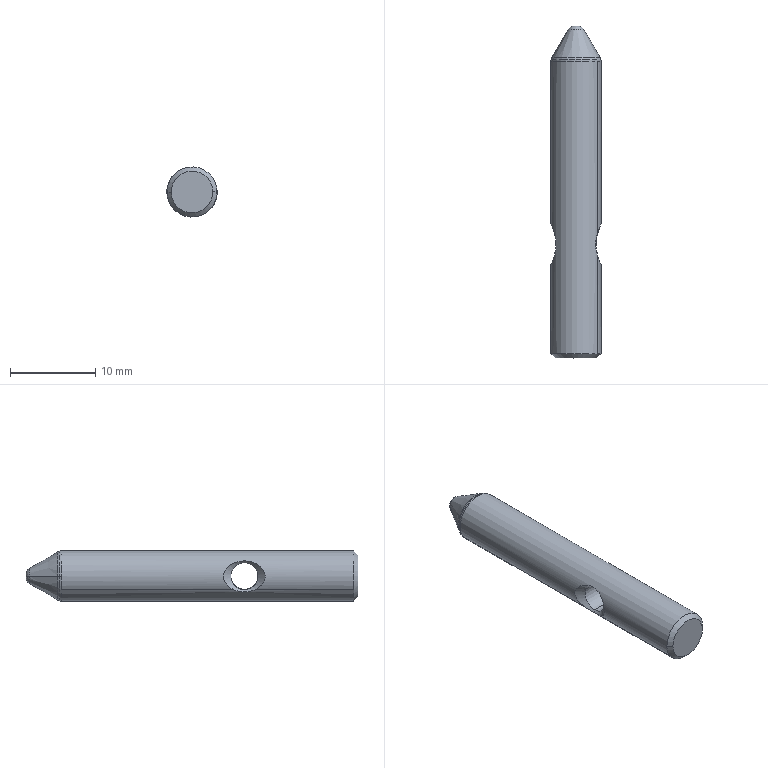Part | NX | features solid 2 | 1 solid | 20 faces | box 5.9 x 39 x 5.9 mm | volume 952.663 mm3 | cone 8 | cylinder 4 | torus 4 | spline 2 | plane 2 | commonest cylinder face diameters 3.2 x2 5.9 x2
STEP:
#1=CARTESIAN_POINT('',(286.395,55.027,28.705));
#2=VERTEX_POINT('',#1);
#3=CARTESIAN_POINT('',(286.206,53.764,28.965));
#4=VERTEX_POINT('',#3);
#5=CARTESIAN_POINT('',(286.395,55.027,28.705));
#6=CARTESIAN_POINT('',(286.283,54.637,28.879));
#7=CARTESIAN_POINT('',(286.206,54.207,28.965));
#8=CARTESIAN_POINT('',(286.206,53.764,28.965));
#9=B_SPLINE_CURVE_WITH_KNOTS('',3,(#5,#6,#7,#8),.UNSPECIFIED.,.F.,.F.,(4,4),(0.,0.001307),.UNSPECIFIED.);
#10=EDGE_CURVE('',#2,#4,#9,.T.);
#11=ORIENTED_EDGE('',*,*,#10,.F.);
#12=CARTESIAN_POINT('',(286.395,75.273,28.705));
#13=VERTEX_POINT('',#12);
#14=CARTESIAN_POINT('',(286.395,51.692,28.705));
#15=DIRECTION('',(0.,-1.,0.));
#16=VECTOR('',#15,1000.);
#17=LINE('',#14,#16);
#18=EDGE_CURVE('',#13,#2,#17,.T.);
#19=ORIENTED_EDGE('',*,*,#18,.F.);
#20=CARTESIAN_POINT('',(280.971,75.273,27.044));
#21=VERTEX_POINT('',#20);
#22=CARTESIAN_POINT('',(283.92,75.273,27.1));
#23=DIRECTION('',(0.,1.,0.));
#24=DIRECTION('',(-0.9998,0.,-0.01902));
#25=AXIS2_PLACEMENT_3D('',#22,#23,#24);
#26=CIRCLE('',#25,2.95);
#27=EDGE_CURVE('',#21,#13,#26,.T.);
#28=ORIENTED_EDGE('',*,*,#27,.F.);
#29=CARTESIAN_POINT('',(281.445,75.273,25.495));
#30=VERTEX_POINT('',#29);
#31=CARTESIAN_POINT('',(283.92,75.273,27.1));
#32=DIRECTION('',(0.,1.,0.));
#33=DIRECTION('',(-0.8391,0.,-0.5441));
#34=AXIS2_PLACEMENT_3D('',#31,#32,#33);
#35=CIRCLE('',#34,2.95);
#36=EDGE_CURVE('',#30,#21,#35,.T.);
#37=ORIENTED_EDGE('',*,*,#36,.F.);
#38=CARTESIAN_POINT('',(281.445,55.027,25.495));
#39=VERTEX_POINT('',#38);
#40=CARTESIAN_POINT('',(281.445,75.273,25.495));
#41=DIRECTION('',(0.000000064,-1.,-0.000000369));
#42=VECTOR('',#41,1000.);
#43=LINE('',#40,#42);
#44=EDGE_CURVE('',#39,#30,#43,.F.);
#45=ORIENTED_EDGE('',*,*,#44,.F.);
#46=CARTESIAN_POINT('',(281.12,55.909,26.17));
#47=VERTEX_POINT('',#46);
#48=CARTESIAN_POINT('',(281.12,55.909,26.17));
#49=CARTESIAN_POINT('',(281.221,55.681,25.866));
#50=CARTESIAN_POINT('',(281.345,55.373,25.649));
#51=CARTESIAN_POINT('',(281.445,55.027,25.495));
#52=B_SPLINE_CURVE_WITH_KNOTS('',3,(#48,#49,#50,#51),.UNSPECIFIED.,.F.,.F.,(4,4),(0.,0.001162),.UNSPECIFIED.);
#53=EDGE_CURVE('',#47,#39,#52,.T.);
#54=ORIENTED_EDGE('',*,*,#53,.F.);
#55=CARTESIAN_POINT('',(281.565,53.764,28.876));
#56=VERTEX_POINT('',#55);
#57=CARTESIAN_POINT('',(281.565,53.764,28.876));
#58=CARTESIAN_POINT('',(281.565,54.133,28.876));
#59=CARTESIAN_POINT('',(281.463,54.856,28.747));
#60=CARTESIAN_POINT('',(281.147,55.78,28.215));
#61=CARTESIAN_POINT('',(280.898,56.363,27.214));
#62=CARTESIAN_POINT('',(281.025,56.124,26.457));
#63=CARTESIAN_POINT('',(281.12,55.909,26.17));
#64=B_SPLINE_CURVE_WITH_KNOTS('',3,(#57,#58,#59,#60,#61,#62,#63),.UNSPECIFIED.,.F.,.F.,(4,1,1,1,4),(0.,0.001091,0.002181,0.003272,0.004362),.UNSPECIFIED.);
#65=EDGE_CURVE('',#56,#47,#64,.T.);
#66=ORIENTED_EDGE('',*,*,#65,.F.);
#67=CARTESIAN_POINT('',(281.445,52.501,25.495));
#68=VERTEX_POINT('',#67);
#69=CARTESIAN_POINT('',(281.445,52.501,25.495));
#70=CARTESIAN_POINT('',(281.326,52.089,25.678));
#71=CARTESIAN_POINT('',(281.091,51.538,26.09));
#72=CARTESIAN_POINT('',(280.941,51.249,27.003));
#73=CARTESIAN_POINT('',(281.033,51.486,27.938));
#74=CARTESIAN_POINT('',(281.399,52.389,28.676));
#75=CARTESIAN_POINT('',(281.565,53.298,28.876));
#76=CARTESIAN_POINT('',(281.565,53.764,28.876));
#77=B_SPLINE_CURVE_WITH_KNOTS('',3,(#69,#70,#71,#72,#73,#74,#75,#76),.UNSPECIFIED.,.F.,.F.,(4,1,1,1,1,4),(0.000000001,0.001379,0.002068,0.002758,0.004136,0.005515),.UNSPECIFIED.);
#78=EDGE_CURVE('',#68,#56,#77,.T.);
#79=ORIENTED_EDGE('',*,*,#78,.F.);
#80=CARTESIAN_POINT('',(281.445,40.924,25.495));
#81=VERTEX_POINT('',#80);
#82=CARTESIAN_POINT('',(281.445,52.501,25.495));
#83=DIRECTION('',(0.000000047,-1.,0.000000146));
#84=VECTOR('',#83,1000.);
#85=LINE('',#82,#84);
#86=EDGE_CURVE('',#81,#68,#85,.F.);
#87=ORIENTED_EDGE('',*,*,#86,.F.);
#88=CARTESIAN_POINT('',(280.971,40.924,27.044));
#89=VERTEX_POINT('',#88);
#90=CARTESIAN_POINT('',(283.92,40.924,27.1));
#91=DIRECTION('',(0.,-1.,0.));
#92=DIRECTION('',(-0.9998,0.,-0.01902));
#93=AXIS2_PLACEMENT_3D('',#90,#91,#92);
#94=CIRCLE('',#93,2.95);
#95=EDGE_CURVE('',#89,#81,#94,.T.);
#96=ORIENTED_EDGE('',*,*,#95,.F.);
#97=CARTESIAN_POINT('',(286.395,40.924,28.705));
#98=VERTEX_POINT('',#97);
#99=CARTESIAN_POINT('',(283.92,40.924,27.1));
#100=DIRECTION('',(0.,-1.,0.));
#101=DIRECTION('',(0.8391,0.,0.5441));
#102=AXIS2_PLACEMENT_3D('',#99,#100,#101);
#103=CIRCLE('',#102,2.95);
#104=EDGE_CURVE('',#98,#89,#103,.T.);
#105=ORIENTED_EDGE('',*,*,#104,.F.);
#106=CARTESIAN_POINT('',(286.395,52.501,28.705));
#107=VERTEX_POINT('',#106);
#108=CARTESIAN_POINT('',(286.395,52.501,28.705));
#109=CARTESIAN_POINT('',(286.395,48.642,28.705));
#110=CARTESIAN_POINT('',(286.395,44.783,28.705));
#111=CARTESIAN_POINT('',(286.395,40.924,28.705));
#112=B_SPLINE_CURVE_WITH_KNOTS('',3,(#108,#109,#110,#111),.UNSPECIFIED.,.F.,.F.,(4,4),(0.,1.),.UNSPECIFIED.);
#113=EDGE_CURVE('',#107,#98,#112,.T.);
#114=ORIENTED_EDGE('',*,*,#113,.F.);
#115=CARTESIAN_POINT('',(286.206,53.764,28.965));
#116=CARTESIAN_POINT('',(286.206,53.322,28.965));
#117=CARTESIAN_POINT('',(286.283,52.891,28.878));
#118=CARTESIAN_POINT('',(286.395,52.501,28.705));
#119=B_SPLINE_CURVE_WITH_KNOTS('',3,(#115,#116,#117,#118),.UNSPECIFIED.,.F.,.F.,(4,4),(0.,0.001308),.UNSPECIFIED.);
#120=EDGE_CURVE('',#4,#107,#119,.T.);
#121=ORIENTED_EDGE('',*,*,#120,.F.);
#122=EDGE_LOOP('',(#11,#19,#28,#37,#45,#54,#66,#79,#87,#96,#105,#114,#121));
#123=FACE_BOUND('',#122,.T.);
#124=CARTESIAN_POINT('',(283.92,51.692,27.1));
#125=DIRECTION('',(0.,-1.,0.));
#126=DIRECTION('',(-0.8391,0.,-0.5441));
#127=AXIS2_PLACEMENT_3D('',#124,#125,#126);
#128=CYLINDRICAL_SURFACE('',#127,2.95);
#129=ADVANCED_FACE('',(#123),#128,.T.);
#130=CARTESIAN_POINT('',(286.05,53.764,25.54));
#131=VERTEX_POINT('',#130);
#132=CARTESIAN_POINT('',(286.275,53.764,25.324));
#133=VERTEX_POINT('',#132);
#134=CARTESIAN_POINT('',(286.05,53.764,25.54));
#135=DIRECTION('',(0.7204,-0.000000028,-0.6935));
#136=VECTOR('',#135,1000.);
#137=LINE('',#134,#136);
#138=EDGE_CURVE('',#131,#133,#137,.T.);
#139=ORIENTED_EDGE('',*,*,#138,.F.);
#140=CARTESIAN_POINT('',(285.989,53.764,28.74));
#141=VERTEX_POINT('',#140);
#142=CARTESIAN_POINT('',(286.02,53.764,27.14));
#143=DIRECTION('',(-0.9998,0.,-0.01902));
#144=DIRECTION('',(0.01902,0.,-0.9998));
#145=AXIS2_PLACEMENT_3D('',#142,#143,#144);
#146=CIRCLE('',#145,1.6);
#147=EDGE_CURVE('',#131,#141,#146,.T.);
#148=ORIENTED_EDGE('',*,*,#147,.T.);
#149=CARTESIAN_POINT('',(285.989,53.764,28.74));
#150=CARTESIAN_POINT('',(286.061,53.764,28.815));
#151=CARTESIAN_POINT('',(286.134,53.764,28.89));
#152=CARTESIAN_POINT('',(286.206,53.764,28.965));
#153=B_SPLINE_CURVE_WITH_KNOTS('',3,(#149,#150,#151,#152),.UNSPECIFIED.,.F.,.F.,(4,4),(0.,0.9998),.UNSPECIFIED.);
#154=EDGE_CURVE('',#4,#141,#153,.F.);
#155=ORIENTED_EDGE('',*,*,#154,.F.);
#156=ORIENTED_EDGE('',*,*,#120,.T.);
#157=CARTESIAN_POINT('',(286.395,52.501,28.705));
#158=CARTESIAN_POINT('',(286.514,52.089,28.521));
#159=CARTESIAN_POINT('',(286.749,51.537,28.109));
#160=CARTESIAN_POINT('',(286.899,51.249,27.197));
#161=CARTESIAN_POINT('',(286.807,51.487,26.262));
#162=CARTESIAN_POINT('',(286.441,52.389,25.524));
#163=CARTESIAN_POINT('',(286.275,53.298,25.324));
#164=CARTESIAN_POINT('',(286.275,53.764,25.324));
#165=B_SPLINE_CURVE_WITH_KNOTS('',3,(#157,#158,#159,#160,#161,#162,#163,#164),.UNSPECIFIED.,.F.,.F.,(4,1,1,1,1,4),(0.,0.001379,0.002068,0.002757,0.004136,0.005514),.UNSPECIFIED.);
#166=EDGE_CURVE('',#107,#133,#165,.T.);
#167=ORIENTED_EDGE('',*,*,#166,.T.);
#168=EDGE_LOOP('',(#139,#148,#155,#156,#167));
#169=FACE_BOUND('',#168,.T.);
#170=CARTESIAN_POINT('',(286.445,53.764,27.148));
#171=DIRECTION('',(0.9998,0.,0.01902));
#172=DIRECTION('',(0.01902,0.,-0.9998));
#173=AXIS2_PLACEMENT_3D('',#170,#171,#172);
#174=CONICAL_SURFACE('',#173,2.025,0.7854);
#175=ADVANCED_FACE('',(#169),#174,.F.);
#176=ORIENTED_EDGE('',*,*,#166,.F.);
#177=ORIENTED_EDGE('',*,*,#113,.T.);
#178=CARTESIAN_POINT('',(286.869,40.924,27.156));
#179=VERTEX_POINT('',#178);
#180=CARTESIAN_POINT('',(283.92,40.924,27.1));
#181=DIRECTION('',(0.,-1.,0.));
#182=DIRECTION('',(0.9998,0.,0.01902));
#183=AXIS2_PLACEMENT_3D('',#180,#181,#182);
#184=CIRCLE('',#183,2.95);
#185=EDGE_CURVE('',#179,#98,#184,.T.);
#186=ORIENTED_EDGE('',*,*,#185,.F.);
#187=CARTESIAN_POINT('',(283.92,40.924,27.1));
#188=DIRECTION('',(0.,-1.,0.));
#189=DIRECTION('',(-0.8391,0.,-0.5441));
#190=AXIS2_PLACEMENT_3D('',#187,#188,#189);
#191=CIRCLE('',#190,2.95);
#192=EDGE_CURVE('',#81,#179,#191,.T.);
#193=ORIENTED_EDGE('',*,*,#192,.F.);
#194=ORIENTED_EDGE('',*,*,#86,.T.);
#195=CARTESIAN_POINT('',(281.634,53.764,25.235));
#196=VERTEX_POINT('',#195);
#197=CARTESIAN_POINT('',(281.634,53.764,25.235));
#198=CARTESIAN_POINT('',(281.634,53.322,25.235));
#199=CARTESIAN_POINT('',(281.557,52.892,25.321));
#200=CARTESIAN_POINT('',(281.445,52.501,25.495));
#201=B_SPLINE_CURVE_WITH_KNOTS('',3,(#197,#198,#199,#200),.UNSPECIFIED.,.F.,.F.,(4,4),(0.,0.001307),.UNSPECIFIED.);
#202=EDGE_CURVE('',#196,#68,#201,.T.);
#203=ORIENTED_EDGE('',*,*,#202,.F.);
#204=CARTESIAN_POINT('',(281.445,55.027,25.495));
#205=CARTESIAN_POINT('',(281.557,54.637,25.321));
#206=CARTESIAN_POINT('',(281.634,54.207,25.235));
#207=CARTESIAN_POINT('',(281.634,53.764,25.235));
#208=B_SPLINE_CURVE_WITH_KNOTS('',3,(#204,#205,#206,#207),.UNSPECIFIED.,.F.,.F.,(4,4),(0.,0.001307),.UNSPECIFIED.);
#209=EDGE_CURVE('',#39,#196,#208,.T.);
#210=ORIENTED_EDGE('',*,*,#209,.F.);
#211=ORIENTED_EDGE('',*,*,#44,.T.);
#212=CARTESIAN_POINT('',(286.869,75.273,27.156));
#213=VERTEX_POINT('',#212);
#214=CARTESIAN_POINT('',(283.92,75.273,27.1));
#215=DIRECTION('',(0.,1.,0.));
#216=DIRECTION('',(0.9998,0.,0.01902));
#217=AXIS2_PLACEMENT_3D('',#214,#215,#216);
#218=CIRCLE('',#217,2.95);
#219=EDGE_CURVE('',#213,#30,#218,.T.);
#220=ORIENTED_EDGE('',*,*,#219,.F.);
#221=CARTESIAN_POINT('',(283.92,75.273,27.1));
#222=DIRECTION('',(0.,1.,0.));
#223=DIRECTION('',(0.8391,0.,0.5441));
#224=AXIS2_PLACEMENT_3D('',#221,#222,#223);
#225=CIRCLE('',#224,2.95);
#226=EDGE_CURVE('',#13,#213,#225,.T.);
#227=ORIENTED_EDGE('',*,*,#226,.F.);
#228=ORIENTED_EDGE('',*,*,#18,.T.);
#229=CARTESIAN_POINT('',(286.753,55.909,26.277));
#230=VERTEX_POINT('',#229);
#231=CARTESIAN_POINT('',(286.753,55.909,26.277));
#232=CARTESIAN_POINT('',(286.812,56.059,26.48));
#233=CARTESIAN_POINT('',(286.903,56.278,26.957));
#234=CARTESIAN_POINT('',(286.801,56.102,28.021));
#235=CARTESIAN_POINT('',(286.527,55.483,28.502));
#236=CARTESIAN_POINT('',(286.395,55.027,28.705));
#237=B_SPLINE_CURVE_WITH_KNOTS('',3,(#231,#232,#233,#234,#235,#236),.UNSPECIFIED.,.F.,.F.,(4,1,1,4),(0.,0.0007668,0.001534,0.003067),.UNSPECIFIED.);
#238=EDGE_CURVE('',#230,#2,#237,.T.);
#239=ORIENTED_EDGE('',*,*,#238,.F.);
#240=CARTESIAN_POINT('',(286.275,53.764,25.324));
#241=CARTESIAN_POINT('',(286.275,54.6,25.324));
#242=CARTESIAN_POINT('',(286.562,55.423,25.621));
#243=CARTESIAN_POINT('',(286.753,55.909,26.277));
#244=B_SPLINE_CURVE_WITH_KNOTS('',3,(#240,#241,#242,#243),.UNSPECIFIED.,.F.,.F.,(4,4),(0.,0.002472),.UNSPECIFIED.);
#245=EDGE_CURVE('',#133,#230,#244,.T.);
#246=ORIENTED_EDGE('',*,*,#245,.F.);
#247=EDGE_LOOP('',(#176,#177,#186,#193,#194,#203,#210,#211,#220,#227,#228,#239,#246));
#248=FACE_BOUND('',#247,.T.);
#249=CARTESIAN_POINT('',(283.92,51.692,27.1));
#250=DIRECTION('',(0.,-1.,0.));
#251=DIRECTION('',(-0.8391,0.,-0.5441));
#252=AXIS2_PLACEMENT_3D('',#249,#250,#251);
#253=CYLINDRICAL_SURFACE('',#252,2.95);
#254=ADVANCED_FACE('',(#248),#253,.T.);
#255=ORIENTED_EDGE('',*,*,#238,.T.);
#256=ORIENTED_EDGE('',*,*,#10,.T.);
#257=ORIENTED_EDGE('',*,*,#154,.T.);
#258=CARTESIAN_POINT('',(286.02,53.764,27.14));
#259=DIRECTION('',(-0.9998,0.,-0.01902));
#260=DIRECTION('',(-0.01902,0.,0.9998));
#261=AXIS2_PLACEMENT_3D('',#258,#259,#260);
#262=CIRCLE('',#261,1.6);
#263=EDGE_CURVE('',#141,#131,#262,.T.);
#264=ORIENTED_EDGE('',*,*,#263,.T.);
#265=ORIENTED_EDGE('',*,*,#138,.T.);
#266=ORIENTED_EDGE('',*,*,#245,.T.);
#267=EDGE_LOOP('',(#255,#256,#257,#264,#265,#266));
#268=FACE_BOUND('',#267,.T.);
#269=CARTESIAN_POINT('',(286.445,53.764,27.148));
#270=DIRECTION('',(0.9998,0.,0.01902));
#271=DIRECTION('',(0.01902,0.,-0.9998));
#272=AXIS2_PLACEMENT_3D('',#269,#270,#271);
#273=CONICAL_SURFACE('',#272,2.025,0.7854);
#274=ADVANCED_FACE('',(#268),#273,.F.);
#275=CARTESIAN_POINT('',(281.79,53.764,28.66));
#276=VERTEX_POINT('',#275);
#277=CARTESIAN_POINT('',(285.989,53.764,28.74));
#278=DIRECTION('',(-0.9998,0.,-0.01902));
#279=VECTOR('',#278,1000.);
#280=LINE('',#277,#279);
#281=EDGE_CURVE('',#141,#276,#280,.T.);
#282=ORIENTED_EDGE('',*,*,#281,.T.);
#283=CARTESIAN_POINT('',(281.851,53.764,25.46));
#284=VERTEX_POINT('',#283);
#285=CARTESIAN_POINT('',(281.82,53.764,27.06));
#286=DIRECTION('',(0.9998,0.,0.01902));
#287=DIRECTION('',(0.01902,0.,-0.9998));
#288=AXIS2_PLACEMENT_3D('',#285,#286,#287);
#289=CIRCLE('',#288,1.6);
#290=EDGE_CURVE('',#284,#276,#289,.T.);
#291=ORIENTED_EDGE('',*,*,#290,.F.);
#292=CARTESIAN_POINT('',(286.05,53.764,25.54));
#293=DIRECTION('',(-0.9998,0.,-0.01902));
#294=VECTOR('',#293,1000.);
#295=LINE('',#292,#294);
#296=EDGE_CURVE('',#284,#131,#295,.F.);
#297=ORIENTED_EDGE('',*,*,#296,.T.);
#298=ORIENTED_EDGE('',*,*,#263,.F.);
#299=EDGE_LOOP('',(#282,#291,#297,#298));
#300=FACE_BOUND('',#299,.T.);
#301=CARTESIAN_POINT('',(288.919,53.764,27.195));
#302=DIRECTION('',(-0.9998,0.,-0.01902));
#303=DIRECTION('',(-0.01902,0.,0.9998));
#304=AXIS2_PLACEMENT_3D('',#301,#302,#303);
#305=CYLINDRICAL_SURFACE('',#304,1.6);
#306=ADVANCED_FACE('',(#300),#305,.F.);
#307=ORIENTED_EDGE('',*,*,#296,.F.);
#308=CARTESIAN_POINT('',(281.82,53.764,27.06));
#309=DIRECTION('',(0.9998,0.,0.01902));
#310=DIRECTION('',(-0.01902,0.,0.9998));
#311=AXIS2_PLACEMENT_3D('',#308,#309,#310);
#312=CIRCLE('',#311,1.6);
#313=EDGE_CURVE('',#276,#284,#312,.T.);
#314=ORIENTED_EDGE('',*,*,#313,.F.);
#315=ORIENTED_EDGE('',*,*,#281,.F.);
#316=ORIENTED_EDGE('',*,*,#147,.F.);
#317=EDGE_LOOP('',(#307,#314,#315,#316));
#318=FACE_BOUND('',#317,.T.);
#319=CARTESIAN_POINT('',(288.919,53.764,27.195));
#320=DIRECTION('',(-0.9998,0.,-0.01902));
#321=DIRECTION('',(-0.01902,0.,0.9998));
#322=AXIS2_PLACEMENT_3D('',#319,#320,#321);
#323=CYLINDRICAL_SURFACE('',#322,1.6);
#324=ADVANCED_FACE('',(#318),#323,.F.);
#325=ORIENTED_EDGE('',*,*,#78,.T.);
#326=CARTESIAN_POINT('',(281.79,53.764,28.66));
#327=CARTESIAN_POINT('',(281.715,53.764,28.732));
#328=CARTESIAN_POINT('',(281.65,53.764,28.795));
#329=CARTESIAN_POINT('',(281.565,53.764,28.876));
#330=B_SPLINE_CURVE_WITH_KNOTS('',3,(#326,#327,#328,#329),.UNSPECIFIED.,.F.,.F.,(4,4),(0.,0.9999),.UNSPECIFIED.);
#331=EDGE_CURVE('',#276,#56,#330,.T.);
#332=ORIENTED_EDGE('',*,*,#331,.F.);
#333=ORIENTED_EDGE('',*,*,#313,.T.);
#334=CARTESIAN_POINT('',(281.851,53.764,25.46));
#335=CARTESIAN_POINT('',(281.779,53.764,25.385));
#336=CARTESIAN_POINT('',(281.706,53.764,25.31));
#337=CARTESIAN_POINT('',(281.634,53.764,25.235));
#338=B_SPLINE_CURVE_WITH_KNOTS('',3,(#334,#335,#336,#337),.UNSPECIFIED.,.F.,.F.,(4,4),(0.,0.9996),.UNSPECIFIED.);
#339=EDGE_CURVE('',#196,#284,#338,.F.);
#340=ORIENTED_EDGE('',*,*,#339,.F.);
#341=ORIENTED_EDGE('',*,*,#202,.T.);
#342=EDGE_LOOP('',(#325,#332,#333,#340,#341));
#343=FACE_BOUND('',#342,.T.);
#344=CARTESIAN_POINT('',(281.395,53.764,27.052));
#345=DIRECTION('',(-0.9998,0.,-0.01902));
#346=DIRECTION('',(-0.01902,0.,0.9998));
#347=AXIS2_PLACEMENT_3D('',#344,#345,#346);
#348=CONICAL_SURFACE('',#347,2.025,0.7854);
#349=ADVANCED_FACE('',(#343),#348,.F.);
#350=ORIENTED_EDGE('',*,*,#209,.T.);
#351=ORIENTED_EDGE('',*,*,#339,.T.);
#352=ORIENTED_EDGE('',*,*,#290,.T.);
#353=ORIENTED_EDGE('',*,*,#331,.T.);
#354=ORIENTED_EDGE('',*,*,#65,.T.);
#355=ORIENTED_EDGE('',*,*,#53,.T.);
#356=EDGE_LOOP('',(#350,#351,#352,#353,#354,#355));
#357=FACE_BOUND('',#356,.T.);
#358=CARTESIAN_POINT('',(281.395,53.764,27.052));
#359=DIRECTION('',(-0.9998,0.,-0.01902));
#360=DIRECTION('',(-0.01902,0.,0.9998));
#361=AXIS2_PLACEMENT_3D('',#358,#359,#360);
#362=CONICAL_SURFACE('',#361,2.025,0.7854);
#363=ADVANCED_FACE('',(#357),#362,.F.);
#364=ORIENTED_EDGE('',*,*,#226,.T.);
#365=CARTESIAN_POINT('',(286.842,75.48,27.156));
#366=VERTEX_POINT('',#365);
#367=CARTESIAN_POINT('',(286.07,75.273,27.141));
#368=DIRECTION('',(-0.01902,0.,0.9998));
#369=DIRECTION('',(0.9998,0.,0.01902));
#370=AXIS2_PLACEMENT_3D('',#367,#368,#369);
#371=CIRCLE('',#370,0.8);
#372=EDGE_CURVE('',#366,#213,#371,.F.);
#373=ORIENTED_EDGE('',*,*,#372,.F.);
#374=CARTESIAN_POINT('',(280.998,75.48,27.044));
#375=VERTEX_POINT('',#374);
#376=CARTESIAN_POINT('',(283.92,75.48,27.1));
#377=DIRECTION('',(0.,1.,0.));
#378=DIRECTION('',(-0.9998,0.,-0.01902));
#379=AXIS2_PLACEMENT_3D('',#376,#377,#378);
#380=CIRCLE('',#379,2.923);
#381=EDGE_CURVE('',#375,#366,#380,.T.);
#382=ORIENTED_EDGE('',*,*,#381,.F.);
#383=CARTESIAN_POINT('',(281.77,75.273,27.059));
#384=DIRECTION('',(0.01902,0.,-0.9998));
#385=DIRECTION('',(-0.9998,0.,-0.01902));
#386=AXIS2_PLACEMENT_3D('',#383,#384,#385);
#387=CIRCLE('',#386,0.8);
#388=EDGE_CURVE('',#21,#375,#387,.T.);
#389=ORIENTED_EDGE('',*,*,#388,.F.);
#390=ORIENTED_EDGE('',*,*,#27,.T.);
#391=EDGE_LOOP('',(#364,#373,#382,#389,#390));
#392=FACE_BOUND('',#391,.T.);
#393=CARTESIAN_POINT('',(283.92,75.273,27.1));
#394=DIRECTION('',(0.,1.,0.));
#395=DIRECTION('',(0.9998,0.,0.01902));
#396=AXIS2_PLACEMENT_3D('',#393,#394,#395);
#397=TOROIDAL_SURFACE('',#396,2.15,0.8);
#398=ADVANCED_FACE('',(#392),#397,.T.);
#399=ORIENTED_EDGE('',*,*,#36,.T.);
#400=ORIENTED_EDGE('',*,*,#388,.T.);
#401=CARTESIAN_POINT('',(283.92,75.48,27.1));
#402=DIRECTION('',(0.,1.,0.));
#403=DIRECTION('',(0.9998,0.,0.01902));
#404=AXIS2_PLACEMENT_3D('',#401,#402,#403);
#405=CIRCLE('',#404,2.923);
#406=EDGE_CURVE('',#366,#375,#405,.T.);
#407=ORIENTED_EDGE('',*,*,#406,.F.);
#408=ORIENTED_EDGE('',*,*,#372,.T.);
#409=ORIENTED_EDGE('',*,*,#219,.T.);
#410=EDGE_LOOP('',(#399,#400,#407,#408,#409));
#411=FACE_BOUND('',#410,.T.);
#412=CARTESIAN_POINT('',(283.92,75.273,27.1));
#413=DIRECTION('',(0.,1.,0.));
#414=DIRECTION('',(0.9998,0.,0.01902));
#415=AXIS2_PLACEMENT_3D('',#412,#413,#414);
#416=TOROIDAL_SURFACE('',#415,2.15,0.8);
#417=ADVANCED_FACE('',(#411),#416,.T.);
#418=CARTESIAN_POINT('',(286.762,75.673,27.154));
#419=VERTEX_POINT('',#418);
#420=CARTESIAN_POINT('',(286.07,75.273,27.141));
#421=DIRECTION('',(-0.01902,0.,0.9998));
#422=DIRECTION('',(0.9658,0.2588,0.01837));
#423=AXIS2_PLACEMENT_3D('',#420,#421,#422);
#424=CIRCLE('',#423,0.8);
#425=EDGE_CURVE('',#366,#419,#424,.T.);
#426=ORIENTED_EDGE('',*,*,#425,.F.);
#427=ORIENTED_EDGE('',*,*,#406,.T.);
#428=CARTESIAN_POINT('',(281.078,75.673,27.046));
#429=VERTEX_POINT('',#428);
#430=CARTESIAN_POINT('',(281.77,75.273,27.059));
#431=DIRECTION('',(0.01902,0.,-0.9998));
#432=DIRECTION('',(-0.9658,0.2588,-0.01837));
#433=AXIS2_PLACEMENT_3D('',#430,#431,#432);
#434=CIRCLE('',#433,0.8);
#435=EDGE_CURVE('',#429,#375,#434,.F.);
#436=ORIENTED_EDGE('',*,*,#435,.F.);
#437=CARTESIAN_POINT('',(283.92,75.673,27.1));
#438=DIRECTION('',(0.,-1.,0.));
#439=DIRECTION('',(-0.9998,0.,-0.01902));
#440=AXIS2_PLACEMENT_3D('',#437,#438,#439);
#441=CIRCLE('',#440,2.843);
#442=EDGE_CURVE('',#429,#419,#441,.T.);
#443=ORIENTED_EDGE('',*,*,#442,.T.);
#444=EDGE_LOOP('',(#426,#427,#436,#443));
#445=FACE_BOUND('',#444,.T.);
#446=CARTESIAN_POINT('',(283.92,75.273,27.1));
#447=DIRECTION('',(0.,1.,0.));
#448=DIRECTION('',(0.9998,0.,0.01902));
#449=AXIS2_PLACEMENT_3D('',#446,#447,#448);
#450=TOROIDAL_SURFACE('',#449,2.15,0.8);
#451=ADVANCED_FACE('',(#445),#450,.T.);
#452=CARTESIAN_POINT('',(284.828,79.024,27.117));
#453=VERTEX_POINT('',#452);
#454=CARTESIAN_POINT('',(284.828,79.024,27.117));
#455=DIRECTION('',(0.4999,-0.866,0.009508));
#456=VECTOR('',#455,1000.);
#457=LINE('',#454,#456);
#458=EDGE_CURVE('',#453,#419,#457,.T.);
#459=ORIENTED_EDGE('',*,*,#458,.T.);
#460=ORIENTED_EDGE('',*,*,#442,.F.);
#461=CARTESIAN_POINT('',(283.012,79.024,27.083));
#462=VERTEX_POINT('',#461);
#463=CARTESIAN_POINT('',(283.012,79.024,27.083));
#464=DIRECTION('',(-0.4999,-0.866,-0.009508));
#465=VECTOR('',#464,1000.);
#466=LINE('',#463,#465);
#467=EDGE_CURVE('',#429,#462,#466,.F.);
#468=ORIENTED_EDGE('',*,*,#467,.T.);
#469=CARTESIAN_POINT('',(283.92,79.024,27.1));
#470=DIRECTION('',(0.,1.,0.));
#471=DIRECTION('',(0.9998,0.,0.01902));
#472=AXIS2_PLACEMENT_3D('',#469,#470,#471);
#473=CIRCLE('',#472,0.9079);
#474=EDGE_CURVE('',#453,#462,#473,.T.);
#475=ORIENTED_EDGE('',*,*,#474,.F.);
#476=EDGE_LOOP('',(#459,#460,#468,#475));
#477=FACE_BOUND('',#476,.T.);
#478=CARTESIAN_POINT('',(283.92,77.349,27.1));
#479=DIRECTION('',(0.,-1.,0.));
#480=DIRECTION('',(-0.9998,0.,-0.01902));
#481=AXIS2_PLACEMENT_3D('',#478,#479,#480);
#482=CONICAL_SURFACE('',#481,1.875,0.5236);
#483=ADVANCED_FACE('',(#477),#482,.T.);
#484=CARTESIAN_POINT('',(283.705,79.424,27.096));
#485=VERTEX_POINT('',#484);
#486=CARTESIAN_POINT('',(283.705,78.624,27.096));
#487=DIRECTION('',(-0.01902,0.,0.9998));
#488=DIRECTION('',(0.,1.,0.));
#489=AXIS2_PLACEMENT_3D('',#486,#487,#488);
#490=CIRCLE('',#489,0.8);
#491=EDGE_CURVE('',#462,#485,#490,.F.);
#492=ORIENTED_EDGE('',*,*,#491,.T.);
#493=CARTESIAN_POINT('',(284.135,79.424,27.104));
#494=VERTEX_POINT('',#493);
#495=CARTESIAN_POINT('',(283.92,79.424,27.1));
#496=DIRECTION('',(0.,1.,0.));
#497=DIRECTION('',(0.9998,0.,0.01902));
#498=AXIS2_PLACEMENT_3D('',#495,#496,#497);
#499=CIRCLE('',#498,0.215);
#500=EDGE_CURVE('',#494,#485,#499,.T.);
#501=ORIENTED_EDGE('',*,*,#500,.F.);
#502=CARTESIAN_POINT('',(284.135,78.624,27.104));
#503=DIRECTION('',(0.01902,0.,-0.9998));
#504=DIRECTION('',(0.,1.,0.));
#505=AXIS2_PLACEMENT_3D('',#502,#503,#504);
#506=CIRCLE('',#505,0.8);
#507=EDGE_CURVE('',#494,#453,#506,.T.);
#508=ORIENTED_EDGE('',*,*,#507,.T.);
#509=ORIENTED_EDGE('',*,*,#474,.T.);
#510=EDGE_LOOP('',(#492,#501,#508,#509));
#511=FACE_BOUND('',#510,.T.);
#512=CARTESIAN_POINT('',(283.757,79.423,27.134));
#513=CARTESIAN_POINT('',(283.434,79.443,27.201));
#514=CARTESIAN_POINT('',(283.153,79.278,27.259));
#515=CARTESIAN_POINT('',(283.009,78.982,27.29));
#516=CARTESIAN_POINT('',(283.733,79.423,27.02));
#517=CARTESIAN_POINT('',(283.363,79.443,26.863));
#518=CARTESIAN_POINT('',(283.042,79.278,26.726));
#519=CARTESIAN_POINT('',(282.877,78.982,26.656));
#520=CARTESIAN_POINT('',(283.807,79.423,26.931));
#521=CARTESIAN_POINT('',(283.584,79.443,26.597));
#522=CARTESIAN_POINT('',(283.39,79.278,26.307));
#523=CARTESIAN_POINT('',(283.29,78.982,26.157));
#524=CARTESIAN_POINT('',(283.923,79.423,26.933));
#525=CARTESIAN_POINT('',(283.929,79.443,26.603));
#526=CARTESIAN_POINT('',(283.935,79.278,26.317));
#527=CARTESIAN_POINT('',(283.938,78.982,26.169));
#528=CARTESIAN_POINT('',(284.039,79.423,26.935));
#529=CARTESIAN_POINT('',(284.275,79.443,26.61));
#530=CARTESIAN_POINT('',(284.48,79.278,26.328));
#531=CARTESIAN_POINT('',(284.585,78.982,26.182));
#532=CARTESIAN_POINT('',(284.11,79.423,27.027));
#533=CARTESIAN_POINT('',(284.485,79.443,26.884));
#534=CARTESIAN_POINT('',(284.811,79.278,26.76));
#535=CARTESIAN_POINT('',(284.979,78.982,26.696));
#536=CARTESIAN_POINT('',(284.082,79.423,27.14));
#537=CARTESIAN_POINT('',(284.402,79.443,27.22));
#538=CARTESIAN_POINT('',(284.68,79.278,27.288));
#539=CARTESIAN_POINT('',(284.823,78.982,27.324));
#540=(BOUNDED_SURFACE()B_SPLINE_SURFACE(3,3,((#512,#513,#514,#515),(#516,#517,#518,#519),(#520,#521,#522,#523),(#524,#525,#526,#527),(#528,#529,#530,#531),(#532,#533,#534,#535),(#536,#537,#538,#539)),.UNSPECIFIED.,.F.,.F.,.F.)B_SPLINE_SURFACE_WITH_KNOTS((4,3,4),(4,4),(0.,0.5,1.),(0.,1.),.PIECEWISE_BEZIER_KNOTS.)GEOMETRIC_REPRESENTATION_ITEM()RATIONAL_B_SPLINE_SURFACE(((1.343,1.195,1.195,1.343),(1.006,0.8949,0.8949,1.006),(1.006,0.8949,0.8949,1.006),(1.343,1.195,1.195,1.343),(1.006,0.8949,0.8949,1.006),(1.006,0.8949,0.8949,1.006),(1.343,1.195,1.195,1.343)))REPRESENTATION_ITEM('')SURFACE());
#541=ADVANCED_FACE('',(#511),#540,.T.);
#542=ORIENTED_EDGE('',*,*,#507,.F.);
#543=CARTESIAN_POINT('',(283.92,79.424,27.1));
#544=DIRECTION('',(0.,1.,0.));
#545=DIRECTION('',(-0.9998,0.,-0.01902));
#546=AXIS2_PLACEMENT_3D('',#543,#544,#545);
#547=CIRCLE('',#546,0.215);
#548=EDGE_CURVE('',#485,#494,#547,.T.);
#549=ORIENTED_EDGE('',*,*,#548,.F.);
#550=ORIENTED_EDGE('',*,*,#491,.F.);
#551=CARTESIAN_POINT('',(283.92,79.024,27.1));
#552=DIRECTION('',(0.,1.,0.));
#553=DIRECTION('',(-0.9998,0.,-0.01902));
#554=AXIS2_PLACEMENT_3D('',#551,#552,#553);
#555=CIRCLE('',#554,0.9079);
#556=EDGE_CURVE('',#462,#453,#555,.T.);
#557=ORIENTED_EDGE('',*,*,#556,.T.);
#558=EDGE_LOOP('',(#542,#549,#550,#557));
#559=FACE_BOUND('',#558,.T.);
#560=CARTESIAN_POINT('',(284.083,79.423,27.066));
#561=CARTESIAN_POINT('',(284.406,79.443,26.999));
#562=CARTESIAN_POINT('',(284.687,79.278,26.941));
#563=CARTESIAN_POINT('',(284.831,78.982,26.91));
#564=CARTESIAN_POINT('',(284.107,79.423,27.18));
#565=CARTESIAN_POINT('',(284.477,79.443,27.337));
#566=CARTESIAN_POINT('',(284.798,79.278,27.474));
#567=CARTESIAN_POINT('',(284.963,78.982,27.544));
#568=CARTESIAN_POINT('',(284.033,79.423,27.269));
#569=CARTESIAN_POINT('',(284.256,79.443,27.603));
#570=CARTESIAN_POINT('',(284.45,79.278,27.893));
#571=CARTESIAN_POINT('',(284.55,78.982,28.043));
#572=CARTESIAN_POINT('',(283.917,79.423,27.267));
#573=CARTESIAN_POINT('',(283.911,79.443,27.597));
#574=CARTESIAN_POINT('',(283.905,79.278,27.883));
#575=CARTESIAN_POINT('',(283.902,78.982,28.031));
#576=CARTESIAN_POINT('',(283.801,79.423,27.265));
#577=CARTESIAN_POINT('',(283.565,79.443,27.59));
#578=CARTESIAN_POINT('',(283.36,79.278,27.872));
#579=CARTESIAN_POINT('',(283.255,78.982,28.018));
#580=CARTESIAN_POINT('',(283.73,79.423,27.173));
#581=CARTESIAN_POINT('',(283.355,79.443,27.316));
#582=CARTESIAN_POINT('',(283.029,79.278,27.44));
#583=CARTESIAN_POINT('',(282.861,78.982,27.504));
#584=CARTESIAN_POINT('',(283.758,79.423,27.06));
#585=CARTESIAN_POINT('',(283.438,79.443,26.98));
#586=CARTESIAN_POINT('',(283.16,79.278,26.912));
#587=CARTESIAN_POINT('',(283.017,78.982,26.876));
#588=(BOUNDED_SURFACE()B_SPLINE_SURFACE(3,3,((#560,#561,#562,#563),(#564,#565,#566,#567),(#568,#569,#570,#571),(#572,#573,#574,#575),(#576,#577,#578,#579),(#580,#581,#582,#583),(#584,#585,#586,#587)),.UNSPECIFIED.,.F.,.F.,.F.)B_SPLINE_SURFACE_WITH_KNOTS((4,3,4),(4,4),(0.,0.5,1.),(0.,1.),.PIECEWISE_BEZIER_KNOTS.)GEOMETRIC_REPRESENTATION_ITEM()RATIONAL_B_SPLINE_SURFACE(((1.343,1.195,1.195,1.343),(1.006,0.8949,0.8949,1.006),(1.006,0.8949,0.8949,1.006),(1.343,1.195,1.195,1.343),(1.006,0.8949,0.8949,1.006),(1.006,0.8949,0.8949,1.006),(1.343,1.195,1.195,1.343)))REPRESENTATION_ITEM('')SURFACE());
#589=ADVANCED_FACE('',(#559),#588,.T.);
#590=ORIENTED_EDGE('',*,*,#467,.F.);
#591=CARTESIAN_POINT('',(283.92,75.673,27.1));
#592=DIRECTION('',(0.,-1.,0.));
#593=DIRECTION('',(0.9998,0.,0.01902));
#594=AXIS2_PLACEMENT_3D('',#591,#592,#593);
#595=CIRCLE('',#594,2.843);
#596=EDGE_CURVE('',#419,#429,#595,.T.);
#597=ORIENTED_EDGE('',*,*,#596,.F.);
#598=ORIENTED_EDGE('',*,*,#458,.F.);
#599=ORIENTED_EDGE('',*,*,#556,.F.);
#600=EDGE_LOOP('',(#590,#597,#598,#599));
#601=FACE_BOUND('',#600,.T.);
#602=CARTESIAN_POINT('',(283.92,77.349,27.1));
#603=DIRECTION('',(0.,-1.,0.));
#604=DIRECTION('',(-0.9998,0.,-0.01902));
#605=AXIS2_PLACEMENT_3D('',#602,#603,#604);
#606=CONICAL_SURFACE('',#605,1.875,0.5236);
#607=ADVANCED_FACE('',(#601),#606,.T.);
#608=ORIENTED_EDGE('',*,*,#435,.T.);
#609=ORIENTED_EDGE('',*,*,#381,.T.);
#610=ORIENTED_EDGE('',*,*,#425,.T.);
#611=ORIENTED_EDGE('',*,*,#596,.T.);
#612=EDGE_LOOP('',(#608,#609,#610,#611));
#613=FACE_BOUND('',#612,.T.);
#614=CARTESIAN_POINT('',(283.92,75.273,27.1));
#615=DIRECTION('',(0.,1.,0.));
#616=DIRECTION('',(0.9998,0.,0.01902));
#617=AXIS2_PLACEMENT_3D('',#614,#615,#616);
#618=TOROIDAL_SURFACE('',#617,2.15,0.8);
#619=ADVANCED_FACE('',(#613),#618,.T.);
#620=ORIENTED_EDGE('',*,*,#500,.T.);
#621=ORIENTED_EDGE('',*,*,#548,.T.);
#622=EDGE_LOOP('',(#620,#621));
#623=FACE_BOUND('',#622,.T.);
#624=CARTESIAN_POINT('',(283.536,79.424,25.301));
#625=DIRECTION('',(0.,1.,0.));
#626=DIRECTION('',(-0.8391,0.,-0.5441));
#627=AXIS2_PLACEMENT_3D('',#624,#625,#626);
#628=PLANE('',#627);
#629=ADVANCED_FACE('',(#623),#628,.T.);
#630=ORIENTED_EDGE('',*,*,#192,.T.);
#631=CARTESIAN_POINT('',(286.37,40.424,27.147));
#632=VERTEX_POINT('',#631);
#633=CARTESIAN_POINT('',(286.37,40.424,27.147));
#634=DIRECTION('',(0.707,0.7071,0.01345));
#635=VECTOR('',#634,1000.);
#636=LINE('',#633,#635);
#637=EDGE_CURVE('',#179,#632,#636,.F.);
#638=ORIENTED_EDGE('',*,*,#637,.T.);
#639=CARTESIAN_POINT('',(281.47,40.424,27.053));
#640=VERTEX_POINT('',#639);
#641=CARTESIAN_POINT('',(283.92,40.424,27.1));
#642=DIRECTION('',(0.,-1.,0.));
#643=DIRECTION('',(-0.9998,0.,-0.01902));
#644=AXIS2_PLACEMENT_3D('',#641,#642,#643);
#645=CIRCLE('',#644,2.45);
#646=EDGE_CURVE('',#640,#632,#645,.T.);
#647=ORIENTED_EDGE('',*,*,#646,.F.);
#648=CARTESIAN_POINT('',(281.47,40.424,27.053));
#649=DIRECTION('',(-0.707,0.7071,-0.01345));
#650=VECTOR('',#649,1000.);
#651=LINE('',#648,#650);
#652=EDGE_CURVE('',#640,#89,#651,.T.);
#653=ORIENTED_EDGE('',*,*,#652,.T.);
#654=ORIENTED_EDGE('',*,*,#95,.T.);
#655=EDGE_LOOP('',(#630,#638,#647,#653,#654));
#656=FACE_BOUND('',#655,.T.);
#657=CARTESIAN_POINT('',(283.92,40.674,27.1));
#658=DIRECTION('',(0.,1.,0.));
#659=DIRECTION('',(0.9998,0.,0.01902));
#660=AXIS2_PLACEMENT_3D('',#657,#658,#659);
#661=CONICAL_SURFACE('',#660,2.7,0.7854);
#662=ADVANCED_FACE('',(#656),#661,.T.);
#663=ORIENTED_EDGE('',*,*,#104,.T.);
#664=ORIENTED_EDGE('',*,*,#652,.F.);
#665=CARTESIAN_POINT('',(283.92,40.424,27.1));
#666=DIRECTION('',(0.,-1.,0.));
#667=DIRECTION('',(0.9998,0.,0.01902));
#668=AXIS2_PLACEMENT_3D('',#665,#666,#667);
#669=CIRCLE('',#668,2.45);
#670=EDGE_CURVE('',#632,#640,#669,.T.);
#671=ORIENTED_EDGE('',*,*,#670,.F.);
#672=ORIENTED_EDGE('',*,*,#637,.F.);
#673=ORIENTED_EDGE('',*,*,#185,.T.);
#674=EDGE_LOOP('',(#663,#664,#671,#672,#673));
#675=FACE_BOUND('',#674,.T.);
#676=CARTESIAN_POINT('',(283.92,40.674,27.1));
#677=DIRECTION('',(0.,1.,0.));
#678=DIRECTION('',(0.9998,0.,0.01902));
#679=AXIS2_PLACEMENT_3D('',#676,#677,#678);
#680=CONICAL_SURFACE('',#679,2.7,0.7854);
#681=ADVANCED_FACE('',(#675),#680,.T.);
#682=ORIENTED_EDGE('',*,*,#646,.T.);
#683=ORIENTED_EDGE('',*,*,#670,.T.);
#684=EDGE_LOOP('',(#682,#683));
#685=FACE_BOUND('',#684,.T.);
#686=CARTESIAN_POINT('',(279.3,40.424,28.085));
#687=DIRECTION('',(0.,-1.,0.));
#688=DIRECTION('',(-0.8391,0.,-0.5441));
#689=AXIS2_PLACEMENT_3D('',#686,#687,#688);
#690=PLANE('',#689);
#691=ADVANCED_FACE('',(#685),#690,.T.);
#692=CLOSED_SHELL('',(#129,#175,#254,#274,#306,#324,#349,#363,#398,#417,#451,#483,#541,#589,#607,#619,#629,#662,#681,#691));
#693=MANIFOLD_SOLID_BREP('',#692);
#694=(LENGTH_UNIT()NAMED_UNIT(*)SI_UNIT(.MILLI.,.METRE.));
#695=UNCERTAINTY_MEASURE_WITH_UNIT(LENGTH_MEASURE(0.0508),#694,'','');
#696=(NAMED_UNIT(*)PLANE_ANGLE_UNIT()SI_UNIT($,.RADIAN.));
#697=(NAMED_UNIT(*)SI_UNIT($,.STERADIAN.)SOLID_ANGLE_UNIT());
#698=(GEOMETRIC_REPRESENTATION_CONTEXT(3)GLOBAL_UNCERTAINTY_ASSIGNED_CONTEXT((#695))GLOBAL_UNIT_ASSIGNED_CONTEXT((#694,#696,#697))REPRESENTATION_CONTEXT('',''));
#699=ADVANCED_BREP_SHAPE_REPRESENTATION('',(#693),#698);